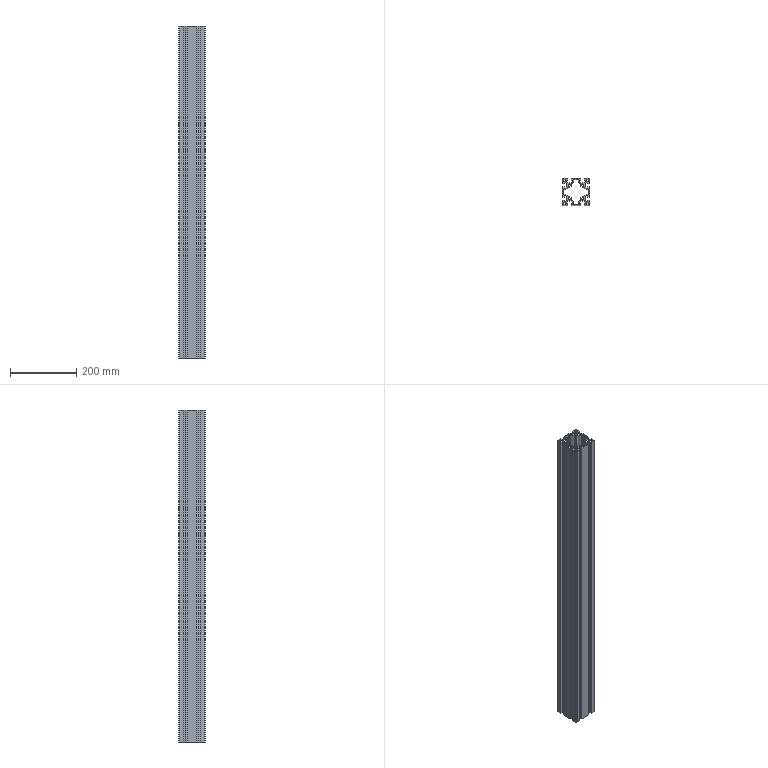Part | SolidWorks | features BaseBody 1 | 1 solid | 236 faces | box 80 x 80 x 1000 mm | volume 1703111 mm3 | plane 154 | cylinder 82 | commonest cylinder face diameters 2 x36 0.6 x20 6.8 x12 12 x10 6 x4